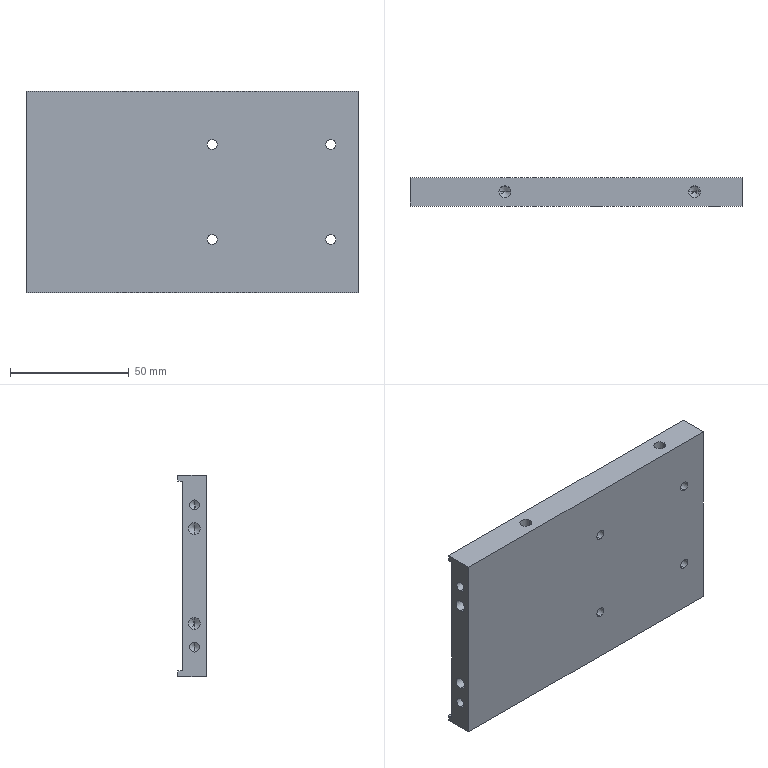Part | STEP file | PN_0029 | 1 solid | 50 faces | box 140 x 12 x 85 mm | volume 117738 mm3 | cylinder 24 | cone 16 | plane 10 | commonest cylinder face diameters 4.2 x12 5 x12